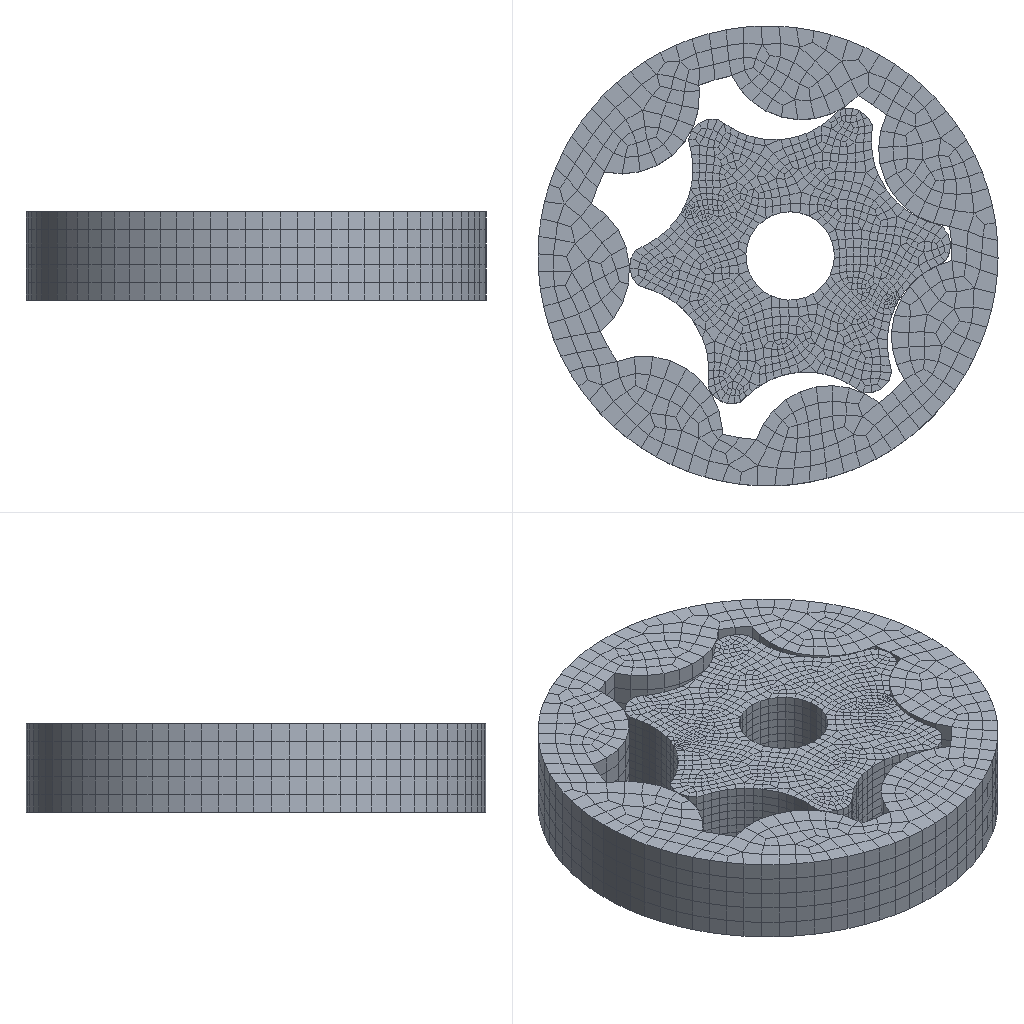Simulation study | abaqus
Set-up summary:
category,name,step,type,value,unit,region
solver,abaqus
solver,version,,,Abaqus/Standard 2020
units,not stated in the deck,,not stated
analysis,deck,,transient,transient
load_step,Step-1,Step-1,transient
load_step,requested,,,1
mesh,nodes,,,14474
mesh,elements,,,11755
element_type,C3D8R,,solid,11755
load,load commands in deck,,count,1
bc,support commands in deck,,count,11
material,MATERIAL-1,,in results
check,setup vs results,,match,"per instance, exact: element labels, types and connectivity; labels of the nodes the elements use; coordinates of those nodes at SINGLE_PRECISION in 2 of 2 instance(s)"
Abaqus input file, long lists of numbers shortened:
*Heading
** Job name: Job-1 Model name: Model-1
** Generated by: Abaqus/CAE 2020
*Preprint, echo=NO, model=NO, history=NO, contact=NO
**
** PARTS
**
*Part, name=part-1
*Node
      1,   24.856,   7.626,           0.
      2,   23.401,   11.331,           0.
** (2734 more lines like these left out)
*Element, type=C3D8R
   1,  278,  282,  243,  200,  734,  738,  699,  656
   2,  383,  195,   31,   32,  839,  651,  487,  488
** (1883 more lines like these left out)
*Node
   2737,           0.,           0.,           5.
*Nset, nset=part-1-RefPt_, internal
2737,
*Nset, nset=Set-1, generate
    1,  2736,     1
*Elset, elset=Set-1, generate
    1,  1885,     1
** Section: Section-1
*Solid Section, elset=Set-1, material=Material-1
,
*End Part
**
*Part, name=part-2
*Node
      1, -0.9005,   3.666,           0.
      2,  0.5733,    4.614,           0.
** (11735 more lines like these left out)
*Element, type=C3D8R
   1,   271,   268,   269,   282,  1338,  1335,  1336,  1349
   2,   223,   220,   204,   208,  1290,  1287,  1271,  1275
** (9868 more lines like these left out)
*Nset, nset=Set-1, generate
     1,  11737,      1
*Elset, elset=Set-1, generate
    1,  9870,     1
** Section: Section-1
*Solid Section, elset=Set-1, material=Material-1
,
*End Part
**
**
** ASSEMBLY
**
*Assembly, name=Assembly
**
*Instance, name=part-1-1, part=part-1
*End Instance
**
*Instance, name=part-2-1, part=part-2
*End Instance
**
*Node
      1,          2.5,           0.,           5.
*Nset, nset=Set-1, instance=part-1-1
    1,    2,    3,    4,    5,    6,    7,    8,    9,   10,   11,   12,   13,   14,   15,   16
   17,   18,   19,   20,   21,   22,   23,   24,   25,   26,   27,   28,   29,   30,   89,   90
** (29 more lines like these left out)
*Elset, elset=Set-1, instance=part-1-1
    3,    4,   14,   22,   32,   43,   50,   56,   58,   59,   68,   69,   75,   80,   82,   85
   94,   95,   96,   97,   99,  100,  101,  103,  104,  105,  107,  108,  109,  110,  111,  113
** (24 more lines like these left out)
*Nset, nset=Set-3
 1,
*Nset, nset=Set-5, instance=part-1-1
 2737,
*Nset, nset=m_Set-2
 1,
*Nset, nset=m_Set-4, instance=part-1-1
 2737,
*Elset, elset=_m_Surf-2_S6, internal, instance=part-2-1
   10,   14,   25,   68,   69,   79,  126,  137,  139,  154,  155,  157,  158,  159,  226,  227
  229,  230,  274,  302,  305,  577,  580,  584,  667,  997, 1001, 1012, 1055, 1056, 1066, 1113
** (14 more lines like these left out)
*Elset, elset=_m_Surf-2_S4, internal, instance=part-2-1
   18,   21,   22,   52,   67,   80,   81,   92,  101,  104,  111,  171,  214,  220,  224,  225
  256,  257,  296,  297,  308,  648,  668,  670,  822,  935,  936,  937,  943, 1005, 1008, 1009
** (17 more lines like these left out)
*Elset, elset=_m_Surf-2_S5, internal, instance=part-2-1
   33,   37,   59,   83,   99,  106,  156,  166,  251,  276,  277,  285,  287,  311,  312,  405
  423,  548,  564,  573,  615,  619,  627,  653,  665,  938,  939,  941, 1020, 1024, 1046, 1070
** (16 more lines like these left out)
*Elset, elset=_m_Surf-2_S3, internal, instance=part-2-1
   11,   19,   23,   24,   50,   65,   66,   75,   84,  109,  110,  129,  160,  190,  191,  228
  375,  438,  440,  479,  485,  499,  515,  519,  520,  531,  551,  556,  559,  560,  563,  571
** (21 more lines like these left out)
*Surface, type=ELEMENT, name=m_Surf-2
_m_Surf-2_S6, S6
_m_Surf-2_S4, S4
_m_Surf-2_S5, S5
_m_Surf-2_S3, S3
*Elset, elset=_s_Surf-1_S6, internal, instance=part-2-1
   36,   56,  116,  135,  162,  422,  435,  448,  491,  522,  523,  566,  611, 1023, 1043, 1103
 1122, 1149, 1409, 1422, 1435, 1478, 1509, 1510, 1553, 1598, 2010, 2030, 2090, 2109, 2136, 2396
** (7 more lines like these left out)
*Elset, elset=_s_Surf-1_S3, internal, instance=part-2-1
   57,  136,  514,  546,  586,  636,  645, 1044, 1123, 1501, 1533, 1573, 1623, 1632, 2031, 2110
 2488, 2520, 2560, 2610, 2619, 3018, 3097, 3475, 3507, 3547, 3597, 3606, 4005, 4084, 4462, 4494
** (3 more lines like these left out)
*Elset, elset=_s_Surf-1_S4, internal, instance=part-2-1
  161,  634,  637,  643, 1148, 1621, 1624, 1630, 2135, 2608, 2611, 2617, 3122, 3595, 3598, 3604
 4109, 4582, 4585, 4591, 5096, 5569, 5572, 5578, 6083, 6556, 6559, 6565, 7070, 7543, 7546, 7552
** (1 more lines like these left out)
*Elset, elset=_s_Surf-1_S5, internal, instance=part-2-1
  165,  447,  492,  524,  635,  641,  655,  719, 1152, 1434, 1479, 1511, 1622, 1628, 1642, 1706
 2139, 2421, 2466, 2498, 2609, 2615, 2629, 2693, 3126, 3408, 3453, 3485, 3596, 3602, 3616, 3680
** (3 more lines like these left out)
*Surface, type=ELEMENT, name=s_Surf-1
_s_Surf-1_S6, S6
_s_Surf-1_S3, S3
_s_Surf-1_S4, S4
_s_Surf-1_S5, S5
*Elset, elset=_s_Surf-2_S5, internal, instance=part-1-1
    2,   11,   24,   28,   36,   37,   39,   44,   49,   63,   71,   77,   79,  130,  134,  139
  140,  144,  146,  151,  156,  162,  164,  166,  173,  175,  187,  189,  268,  270,  271,  278
** (8 more lines like these left out)
*Elset, elset=_s_Surf-2_S6, internal, instance=part-1-1
   55,  143,  153,  198,  261,  432,  520,  530,  575,  638,  809,  897,  907,  952, 1015, 1186
 1274, 1284, 1329, 1392, 1563, 1651, 1661, 1706, 1769
*Elset, elset=_s_Surf-2_S3, internal, instance=part-1-1
    6,   15,   18,   29,   33,   42,   45,   46,   47,   51,   60,   62,   65,   66,   67,   70
   74,   81,   91,  114,  126,  127,  128,  129,  131,  133,  158,  194,  199,  217,  239,  276
** (8 more lines like these left out)
*Elset, elset=_s_Surf-2_S4, internal, instance=part-1-1
   21,   25,  142,  259,  263,  398,  402,  519,  636,  640,  775,  779,  896, 1013, 1017, 1152
 1156, 1273, 1390, 1394, 1529, 1533, 1650, 1767, 1771
*Surface, type=ELEMENT, name=s_Surf-2
_s_Surf-2_S5, S5
_s_Surf-2_S6, S6
_s_Surf-2_S4, S4
_s_Surf-2_S3, S3
*Elset, elset=_s_Surf-4_S6, internal, instance=part-1-1
   14,   22,   43,   56,   59,   75,   82,   85,   95,  101,  104,  105,  107,  108,  113,  136
  145,  152,  185,  186,  216,  221,  255,  391,  399,  420,  433,  436,  452,  459,  462,  472
** (6 more lines like these left out)
*Elset, elset=_s_Surf-4_S4, internal, instance=part-1-1
    4,   32,   50,   58,   69,   80,   94,   96,   97,  100,  109,  110,  141,  190,  192,  195
  197,  200,  201,  206,  208,  209,  211,  212,  219,  222,  223,  227,  228,  230,  231,  232
** (11 more lines like these left out)
*Elset, elset=_s_Surf-4_S5, internal, instance=part-1-1
   68,   99,  103,  111,  181,  188,  191,  203,  224,  226,  245,  258,  445,  476,  480,  488
  558,  565,  568,  580,  601,  603,  622,  635,  822,  853,  857,  865,  935,  942,  945,  957
** (2 more lines like these left out)
*Elset, elset=_s_Surf-4_S3, internal, instance=part-1-1
    3,  119,  124,  138,  169,  174,  380,  496,  501,  515,  546,  551,  757,  873,  878,  892
  923,  928, 1134, 1250, 1255, 1269, 1300, 1305, 1511, 1627, 1632, 1646, 1677, 1682
*Surface, type=ELEMENT, name=s_Surf-4
_s_Surf-4_S6, S6
_s_Surf-4_S4, S4
_s_Surf-4_S5, S5
_s_Surf-4_S3, S3
** Constraint: Constraint-1
*Coupling, constraint name=Constraint-1, ref node=m_Set-2, surface=s_Surf-1
*Kinematic
** Constraint: Constraint-2
*Coupling, constraint name=Constraint-2, ref node=m_Set-4, surface=s_Surf-4
*Kinematic
*End Assembly
*Amplitude, name=Amp-1
             0.,              0.,              1.,              1.
**
** MATERIALS
**
*Material, name=Material-1
*Density
 6.9e-09,
*Elastic
135000., 0.27
*Plastic
350.,0.
**
** INTERACTION PROPERTIES
**
*Surface Interaction, name=IntProp-1
1.,
*Friction, slip tolerance=0.005
 0.2,
*Surface Behavior, pressure-overclosure=HARD
**
** INTERACTIONS
**
** Interaction: Int-1
*Contact Pair, interaction=IntProp-1, type=SURFACE TO SURFACE
s_Surf-2, m_Surf-2
** ----------------------------------------------------------------
**
** STEP: Step-1
**
*Step, name=Step-1, nlgeom=YES, inc=10000
*Dynamic
0.001,1.,1e-05
**
** BOUNDARY CONDITIONS
**
** Name: BC-1 Type: 位移/转角
*Boundary
Set-5, 1, 1
Set-5, 2, 2
Set-5, 3, 3
Set-5, 4, 4
Set-5, 5, 5
** Name: BC-2 Type: 位移/转角
*Boundary, amplitude=Amp-1
Set-3, 1, 1
Set-3, 2, 2
Set-3, 3, 3
Set-3, 4, 4
Set-3, 5, 5
Set-3, 6, 6, -6.28
**
** OUTPUT REQUESTS
**
*Restart, write, frequency=0
**
** FIELD OUTPUT: F-Output-1
**
*Output, field
*Node Output
A, CF, RF, U, V
*Element Output, directions=YES
E, LE, MISES, PE, PEEQ, PEEQMAX, PEEQT, PEMAG, S
*Contact Output
CDISP, CSTRESS
**
** HISTORY OUTPUT: H-Output-1
**
*Output, history, frequency=1
*Node Output, nset=m_Set-2
RF1, RF2, RF3, RM1, RM2, RM3
*End Step
Results summary:
result,step,,partial,increments=406 time=0.1844/1.0
result,analysis,,,transient
result,last_loadstep,,,1
result,primary field,,,U
result,reaction total,,FX,-5e-06,model units
result,reaction total,,FY,7e-06,model units
result,reaction total,,FZ,-0.0,model units